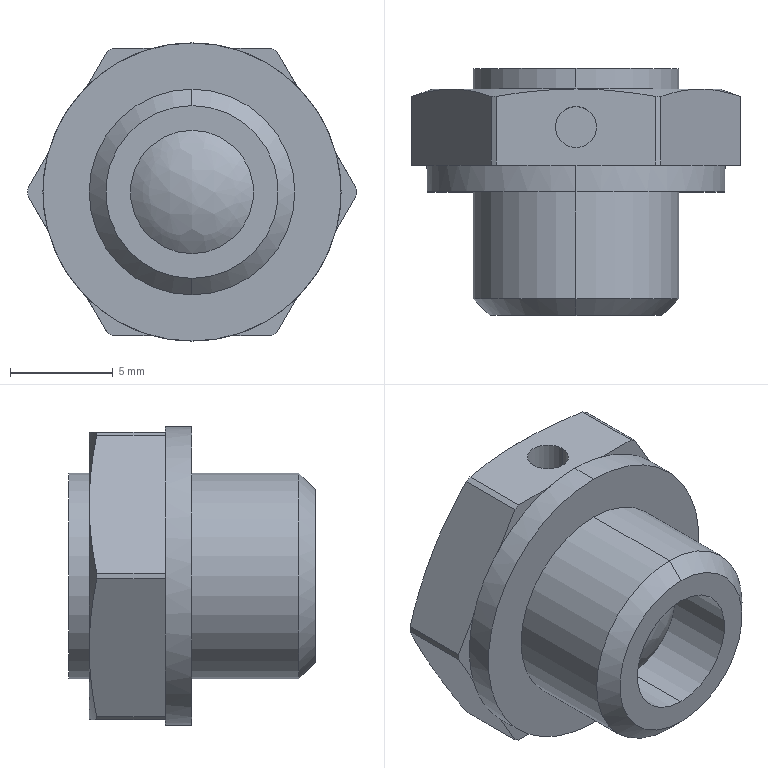Part | SolidWorks | features BaseBody 1 | 1 solid | 49 faces | box 16 x 12 x 14.5 mm | volume 1277 mm3 | plane 23 | cylinder 16 | cone 9 | spline 1 | commonest cylinder face diameters 16 x6 10 x4 2 x2 6 x2 14.5 x2
STEP:
#1=CARTESIAN_POINT('',(0.,0.,-5.));
#2=VERTEX_POINT('',#1);
#3=CARTESIAN_POINT('',(0.,0.,5.));
#4=VERTEX_POINT('',#3);
#5=CARTESIAN_POINT('',(0.,0.,0.));
#6=DIRECTION('',(0.,-1.,0.));
#7=DIRECTION('',(0.,0.,-1.));
#8=AXIS2_PLACEMENT_3D('',#5,#6,#7);
#9=CIRCLE('',#8,5.);
#10=EDGE_CURVE('',#2,#4,#9,.T.);
#11=ORIENTED_EDGE('',*,*,#10,.T.);
#12=CARTESIAN_POINT('',(0.,-5.2,5.));
#13=VERTEX_POINT('',#12);
#14=CARTESIAN_POINT('',(0.,-3.6,5.));
#15=DIRECTION('',(0.,-1.,0.));
#16=VECTOR('',#15,1000.);
#17=LINE('',#14,#16);
#18=EDGE_CURVE('',#4,#13,#17,.T.);
#19=ORIENTED_EDGE('',*,*,#18,.T.);
#20=CARTESIAN_POINT('',(0.,-5.2,-5.));
#21=VERTEX_POINT('',#20);
#22=CARTESIAN_POINT('',(0.,-5.2,0.));
#23=DIRECTION('',(0.,1.,0.));
#24=DIRECTION('',(0.,0.,-1.));
#25=AXIS2_PLACEMENT_3D('',#22,#23,#24);
#26=CIRCLE('',#25,5.);
#27=EDGE_CURVE('',#13,#21,#26,.T.);
#28=ORIENTED_EDGE('',*,*,#27,.T.);
#29=CARTESIAN_POINT('',(0.,-3.6,-5.));
#30=DIRECTION('',(0.,-1.,0.));
#31=VECTOR('',#30,1000.);
#32=LINE('',#29,#31);
#33=EDGE_CURVE('',#2,#21,#32,.T.);
#34=ORIENTED_EDGE('',*,*,#33,.F.);
#35=EDGE_LOOP('',(#11,#19,#28,#34));
#36=FACE_OUTER_BOUND('',#35,.T.);
#37=CARTESIAN_POINT('',(0.,-3.6,0.));
#38=DIRECTION('',(0.,-1.,0.));
#39=DIRECTION('',(0.,0.,-1.));
#40=AXIS2_PLACEMENT_3D('',#37,#38,#39);
#41=CYLINDRICAL_SURFACE('',#40,5.);
#42=ADVANCED_FACE('',(#36),#41,.T.);
#43=CARTESIAN_POINT('',(0.,-6.,4.2));
#44=VERTEX_POINT('',#43);
#45=CARTESIAN_POINT('',(0.,-6.,-4.2));
#46=VERTEX_POINT('',#45);
#47=CARTESIAN_POINT('',(0.,-6.,0.));
#48=DIRECTION('',(0.,1.,0.));
#49=DIRECTION('',(0.,0.,1.));
#50=AXIS2_PLACEMENT_3D('',#47,#48,#49);
#51=CIRCLE('',#50,4.2);
#52=EDGE_CURVE('',#44,#46,#51,.T.);
#53=ORIENTED_EDGE('',*,*,#52,.T.);
#54=CARTESIAN_POINT('',(0.,-5.2,-5.));
#55=DIRECTION('',(0.,0.7071,-0.7071));
#56=VECTOR('',#55,1000.);
#57=LINE('',#54,#56);
#58=EDGE_CURVE('',#46,#21,#57,.T.);
#59=ORIENTED_EDGE('',*,*,#58,.T.);
#60=ORIENTED_EDGE('',*,*,#27,.F.);
#61=CARTESIAN_POINT('',(0.,-5.2,5.));
#62=DIRECTION('',(0.,0.7071,0.7071));
#63=VECTOR('',#62,1000.);
#64=LINE('',#61,#63);
#65=EDGE_CURVE('',#44,#13,#64,.T.);
#66=ORIENTED_EDGE('',*,*,#65,.F.);
#67=EDGE_LOOP('',(#53,#59,#60,#66));
#68=FACE_OUTER_BOUND('',#67,.T.);
#69=CARTESIAN_POINT('',(0.,-5.2,0.));
#70=DIRECTION('',(0.,1.,0.));
#71=DIRECTION('',(0.,0.,1.));
#72=AXIS2_PLACEMENT_3D('',#69,#70,#71);
#73=CONICAL_SURFACE('',#72,5.,0.7854);
#74=ADVANCED_FACE('',(#68),#73,.T.);
#75=CARTESIAN_POINT('',(1.887,1.3,7.));
#76=VERTEX_POINT('',#75);
#77=CARTESIAN_POINT('',(0.,1.3,7.25));
#78=VERTEX_POINT('',#77);
#79=CARTESIAN_POINT('',(0.,1.3,0.));
#80=DIRECTION('',(0.,-1.,0.));
#81=DIRECTION('',(0.,0.,-1.));
#82=AXIS2_PLACEMENT_3D('',#79,#80,#81);
#83=CIRCLE('',#82,7.25);
#84=EDGE_CURVE('',#76,#78,#83,.T.);
#85=ORIENTED_EDGE('',*,*,#84,.T.);
#86=CARTESIAN_POINT('',(0.,0.,7.25));
#87=VERTEX_POINT('',#86);
#88=CARTESIAN_POINT('',(0.,-3.6,7.25));
#89=DIRECTION('',(0.,-1.,0.));
#90=VECTOR('',#89,1000.);
#91=LINE('',#88,#90);
#92=EDGE_CURVE('',#78,#87,#91,.T.);
#93=ORIENTED_EDGE('',*,*,#92,.T.);
#94=CARTESIAN_POINT('',(0.,0.,-7.25));
#95=VERTEX_POINT('',#94);
#96=CARTESIAN_POINT('',(0.,0.,0.));
#97=DIRECTION('',(0.,1.,0.));
#98=DIRECTION('',(0.,0.,-1.));
#99=AXIS2_PLACEMENT_3D('',#96,#97,#98);
#100=CIRCLE('',#99,7.25);
#101=EDGE_CURVE('',#87,#95,#100,.T.);
#102=ORIENTED_EDGE('',*,*,#101,.T.);
#103=CARTESIAN_POINT('',(0.,1.3,-7.25));
#104=VERTEX_POINT('',#103);
#105=CARTESIAN_POINT('',(0.,-3.6,-7.25));
#106=DIRECTION('',(0.,-1.,0.));
#107=VECTOR('',#106,1000.);
#108=LINE('',#105,#107);
#109=EDGE_CURVE('',#104,#95,#108,.T.);
#110=ORIENTED_EDGE('',*,*,#109,.F.);
#111=CARTESIAN_POINT('',(1.887,1.3,-7.));
#112=VERTEX_POINT('',#111);
#113=CARTESIAN_POINT('',(0.,1.3,0.));
#114=DIRECTION('',(0.,-1.,0.));
#115=DIRECTION('',(0.,0.,-1.));
#116=AXIS2_PLACEMENT_3D('',#113,#114,#115);
#117=CIRCLE('',#116,7.25);
#118=EDGE_CURVE('',#104,#112,#117,.T.);
#119=ORIENTED_EDGE('',*,*,#118,.T.);
#120=CARTESIAN_POINT('',(5.118,1.3,-5.135));
#121=VERTEX_POINT('',#120);
#122=CARTESIAN_POINT('',(0.,1.3,0.));
#123=DIRECTION('',(0.,-1.,0.));
#124=DIRECTION('',(0.,0.,-1.));
#125=AXIS2_PLACEMENT_3D('',#122,#123,#124);
#126=CIRCLE('',#125,7.25);
#127=EDGE_CURVE('',#112,#121,#126,.T.);
#128=ORIENTED_EDGE('',*,*,#127,.T.);
#129=CARTESIAN_POINT('',(7.006,1.3,-1.865));
#130=VERTEX_POINT('',#129);
#131=CARTESIAN_POINT('',(0.,1.3,0.));
#132=DIRECTION('',(0.,-1.,0.));
#133=DIRECTION('',(0.,0.,-1.));
#134=AXIS2_PLACEMENT_3D('',#131,#132,#133);
#135=CIRCLE('',#134,7.25);
#136=EDGE_CURVE('',#121,#130,#135,.T.);
#137=ORIENTED_EDGE('',*,*,#136,.T.);
#138=CARTESIAN_POINT('',(7.006,1.3,1.865));
#139=VERTEX_POINT('',#138);
#140=CARTESIAN_POINT('',(0.,1.3,0.));
#141=DIRECTION('',(0.,-1.,0.));
#142=DIRECTION('',(0.,0.,-1.));
#143=AXIS2_PLACEMENT_3D('',#140,#141,#142);
#144=CIRCLE('',#143,7.25);
#145=EDGE_CURVE('',#130,#139,#144,.T.);
#146=ORIENTED_EDGE('',*,*,#145,.T.);
#147=CARTESIAN_POINT('',(5.118,1.3,5.135));
#148=VERTEX_POINT('',#147);
#149=CARTESIAN_POINT('',(0.,1.3,0.));
#150=DIRECTION('',(0.,-1.,0.));
#151=DIRECTION('',(0.,0.,-1.));
#152=AXIS2_PLACEMENT_3D('',#149,#150,#151);
#153=CIRCLE('',#152,7.25);
#154=EDGE_CURVE('',#139,#148,#153,.T.);
#155=ORIENTED_EDGE('',*,*,#154,.T.);
#156=CARTESIAN_POINT('',(0.,1.3,0.));
#157=DIRECTION('',(0.,-1.,0.));
#158=DIRECTION('',(0.,0.,-1.));
#159=AXIS2_PLACEMENT_3D('',#156,#157,#158);
#160=CIRCLE('',#159,7.25);
#161=EDGE_CURVE('',#148,#76,#160,.T.);
#162=ORIENTED_EDGE('',*,*,#161,.T.);
#163=EDGE_LOOP('',(#85,#93,#102,#110,#119,#128,#137,#146,#155,#162));
#164=FACE_OUTER_BOUND('',#163,.T.);
#165=CARTESIAN_POINT('',(0.,-3.6,0.));
#166=DIRECTION('',(0.,-1.,0.));
#167=DIRECTION('',(0.,0.,-1.));
#168=AXIS2_PLACEMENT_3D('',#165,#166,#167);
#169=CYLINDRICAL_SURFACE('',#168,7.25);
#170=ADVANCED_FACE('',(#164),#169,.T.);
#171=CARTESIAN_POINT('',(0.,-2.6,3.));
#172=VERTEX_POINT('',#171);
#173=CARTESIAN_POINT('',(0.,-2.6,-3.));
#174=VERTEX_POINT('',#173);
#175=CARTESIAN_POINT('',(0.,-2.6,0.));
#176=DIRECTION('',(0.,-1.,0.));
#177=DIRECTION('',(0.,0.,-1.));
#178=AXIS2_PLACEMENT_3D('',#175,#176,#177);
#179=CIRCLE('',#178,3.);
#180=EDGE_CURVE('',#172,#174,#179,.T.);
#181=ORIENTED_EDGE('',*,*,#180,.F.);
#182=CARTESIAN_POINT('',(0.,-6.,3.));
#183=VERTEX_POINT('',#182);
#184=CARTESIAN_POINT('',(0.,-3.6,3.));
#185=DIRECTION('',(0.,-1.,0.));
#186=VECTOR('',#185,1000.);
#187=LINE('',#184,#186);
#188=EDGE_CURVE('',#172,#183,#187,.T.);
#189=ORIENTED_EDGE('',*,*,#188,.T.);
#190=CARTESIAN_POINT('',(0.,-6.,-3.));
#191=VERTEX_POINT('',#190);
#192=CARTESIAN_POINT('',(0.,-6.,0.));
#193=DIRECTION('',(0.,-1.,0.));
#194=DIRECTION('',(0.,0.,-1.));
#195=AXIS2_PLACEMENT_3D('',#192,#193,#194);
#196=CIRCLE('',#195,3.);
#197=EDGE_CURVE('',#183,#191,#196,.T.);
#198=ORIENTED_EDGE('',*,*,#197,.T.);
#199=CARTESIAN_POINT('',(0.,-3.6,-3.));
#200=DIRECTION('',(0.,-1.,0.));
#201=VECTOR('',#200,1000.);
#202=LINE('',#199,#201);
#203=EDGE_CURVE('',#174,#191,#202,.T.);
#204=ORIENTED_EDGE('',*,*,#203,.F.);
#205=EDGE_LOOP('',(#181,#189,#198,#204));
#206=FACE_OUTER_BOUND('',#205,.T.);
#207=CARTESIAN_POINT('',(0.,-3.6,0.));
#208=DIRECTION('',(0.,-1.,0.));
#209=DIRECTION('',(0.,0.,-1.));
#210=AXIS2_PLACEMENT_3D('',#207,#208,#209);
#211=CYLINDRICAL_SURFACE('',#210,3.);
#212=ADVANCED_FACE('',(#206),#211,.F.);
#213=CARTESIAN_POINT('',(6.062,5.,-3.5));
#214=VERTEX_POINT('',#213);
#215=CARTESIAN_POINT('',(7.,5.,0.));
#216=VERTEX_POINT('',#215);
#217=CARTESIAN_POINT('',(0.,5.,0.));
#218=DIRECTION('',(0.,-1.,0.));
#219=DIRECTION('',(1.,0.,0.));
#220=AXIS2_PLACEMENT_3D('',#217,#218,#219);
#221=CIRCLE('',#220,7.);
#222=EDGE_CURVE('',#214,#216,#221,.T.);
#223=ORIENTED_EDGE('',*,*,#222,.T.);
#224=CARTESIAN_POINT('',(8.,4.636,0.));
#225=VERTEX_POINT('',#224);
#226=CARTESIAN_POINT('',(8.,4.636,0.));
#227=DIRECTION('',(0.9397,-0.342,0.));
#228=VECTOR('',#227,1000.);
#229=LINE('',#226,#228);
#230=EDGE_CURVE('',#216,#225,#229,.T.);
#231=ORIENTED_EDGE('',*,*,#230,.T.);
#232=CARTESIAN_POINT('',(7.999,4.636,-0.1459));
#233=VERTEX_POINT('',#232);
#234=CARTESIAN_POINT('',(0.,4.636,0.));
#235=DIRECTION('',(0.,-1.,0.));
#236=DIRECTION('',(0.,0.,-1.));
#237=AXIS2_PLACEMENT_3D('',#234,#235,#236);
#238=CIRCLE('',#237,8.);
#239=EDGE_CURVE('',#233,#225,#238,.T.);
#240=ORIENTED_EDGE('',*,*,#239,.F.);
#241=CARTESIAN_POINT('',(7.999,4.636,-0.1459));
#242=CARTESIAN_POINT('',(7.358,4.862,-1.255));
#243=CARTESIAN_POINT('',(6.713,5.,-2.372));
#244=CARTESIAN_POINT('',(6.062,5.,-3.5));
#245=B_SPLINE_CURVE_WITH_KNOTS('',3,(#241,#242,#243,#244),.UNSPECIFIED.,.F.,.F.,(4,4),(0.,0.00389),.UNSPECIFIED.);
#246=EDGE_CURVE('',#233,#214,#245,.T.);
#247=ORIENTED_EDGE('',*,*,#246,.T.);
#248=EDGE_LOOP('',(#223,#231,#240,#247));
#249=FACE_OUTER_BOUND('',#248,.T.);
#250=CARTESIAN_POINT('',(0.,4.636,0.));
#251=DIRECTION('',(0.,-1.,0.));
#252=DIRECTION('',(1.,0.,0.));
#253=AXIS2_PLACEMENT_3D('',#250,#251,#252);
#254=CONICAL_SURFACE('',#253,8.,1.222);
#255=ADVANCED_FACE('',(#249),#254,.T.);
#256=CARTESIAN_POINT('',(-1.,3.15,7.));
#257=VERTEX_POINT('',#256);
#258=CARTESIAN_POINT('',(1.,3.15,7.));
#259=VERTEX_POINT('',#258);
#260=CARTESIAN_POINT('',(0.,3.15,7.));
#261=DIRECTION('',(0.,0.,1.));
#262=DIRECTION('',(-1.,0.,0.));
#263=AXIS2_PLACEMENT_3D('',#260,#261,#262);
#264=CIRCLE('',#263,1.);
#265=EDGE_CURVE('',#257,#259,#264,.T.);
#266=ORIENTED_EDGE('',*,*,#265,.T.);
#267=CARTESIAN_POINT('',(1.,3.15,0.));
#268=VERTEX_POINT('',#267);
#269=CARTESIAN_POINT('',(1.,3.15,0.));
#270=DIRECTION('',(0.,0.,-1.));
#271=VECTOR('',#270,1000.);
#272=LINE('',#269,#271);
#273=EDGE_CURVE('',#259,#268,#272,.T.);
#274=ORIENTED_EDGE('',*,*,#273,.T.);
#275=CARTESIAN_POINT('',(-1.,3.15,0.));
#276=VERTEX_POINT('',#275);
#277=CARTESIAN_POINT('',(0.,3.15,0.));
#278=DIRECTION('',(0.,0.,1.));
#279=DIRECTION('',(-1.,0.,0.));
#280=AXIS2_PLACEMENT_3D('',#277,#278,#279);
#281=CIRCLE('',#280,1.);
#282=EDGE_CURVE('',#276,#268,#281,.T.);
#283=ORIENTED_EDGE('',*,*,#282,.F.);
#284=CARTESIAN_POINT('',(-1.,3.15,0.));
#285=DIRECTION('',(0.,0.,-1.));
#286=VECTOR('',#285,1000.);
#287=LINE('',#284,#286);
#288=EDGE_CURVE('',#257,#276,#287,.T.);
#289=ORIENTED_EDGE('',*,*,#288,.F.);
#290=EDGE_LOOP('',(#266,#274,#283,#289));
#291=FACE_OUTER_BOUND('',#290,.T.);
#292=CARTESIAN_POINT('',(0.,3.15,0.));
#293=DIRECTION('',(0.,0.,-1.));
#294=DIRECTION('',(-1.,0.,0.));
#295=AXIS2_PLACEMENT_3D('',#292,#293,#294);
#296=CYLINDRICAL_SURFACE('',#295,1.);
#297=ADVANCED_FACE('',(#291),#296,.F.);
#298=CARTESIAN_POINT('',(0.,6.,-5.));
#299=VERTEX_POINT('',#298);
#300=CARTESIAN_POINT('',(0.,6.,5.));
#301=VERTEX_POINT('',#300);
#302=CARTESIAN_POINT('',(0.,6.,0.));
#303=DIRECTION('',(0.,-1.,0.));
#304=DIRECTION('',(0.,0.,-1.));
#305=AXIS2_PLACEMENT_3D('',#302,#303,#304);
#306=CIRCLE('',#305,5.);
#307=EDGE_CURVE('',#299,#301,#306,.T.);
#308=ORIENTED_EDGE('',*,*,#307,.T.);
#309=CARTESIAN_POINT('',(0.,5.,5.));
#310=VERTEX_POINT('',#309);
#311=CARTESIAN_POINT('',(0.,-3.6,5.));
#312=DIRECTION('',(0.,-1.,0.));
#313=VECTOR('',#312,1000.);
#314=LINE('',#311,#313);
#315=EDGE_CURVE('',#301,#310,#314,.T.);
#316=ORIENTED_EDGE('',*,*,#315,.T.);
#317=CARTESIAN_POINT('',(0.,5.,-5.));
#318=VERTEX_POINT('',#317);
#319=CARTESIAN_POINT('',(0.,5.,0.));
#320=DIRECTION('',(0.,1.,0.));
#321=DIRECTION('',(0.,0.,-1.));
#322=AXIS2_PLACEMENT_3D('',#319,#320,#321);
#323=CIRCLE('',#322,5.);
#324=EDGE_CURVE('',#310,#318,#323,.T.);
#325=ORIENTED_EDGE('',*,*,#324,.T.);
#326=CARTESIAN_POINT('',(0.,-3.6,-5.));
#327=DIRECTION('',(0.,-1.,0.));
#328=VECTOR('',#327,1000.);
#329=LINE('',#326,#328);
#330=EDGE_CURVE('',#299,#318,#329,.T.);
#331=ORIENTED_EDGE('',*,*,#330,.F.);
#332=EDGE_LOOP('',(#308,#316,#325,#331));
#333=FACE_OUTER_BOUND('',#332,.T.);
#334=CARTESIAN_POINT('',(0.,-3.6,0.));
#335=DIRECTION('',(0.,-1.,0.));
#336=DIRECTION('',(0.,0.,-1.));
#337=AXIS2_PLACEMENT_3D('',#334,#335,#336);
#338=CYLINDRICAL_SURFACE('',#337,5.);
#339=ADVANCED_FACE('',(#333),#338,.T.);
#340=ORIENTED_EDGE('',*,*,#18,.F.);
#341=CARTESIAN_POINT('',(0.,0.,0.));
#342=DIRECTION('',(0.,-1.,0.));
#343=DIRECTION('',(0.,0.,-1.));
#344=AXIS2_PLACEMENT_3D('',#341,#342,#343);
#345=CIRCLE('',#344,5.);
#346=EDGE_CURVE('',#4,#2,#345,.T.);
#347=ORIENTED_EDGE('',*,*,#346,.T.);
#348=ORIENTED_EDGE('',*,*,#33,.T.);
#349=CARTESIAN_POINT('',(0.,-5.2,0.));
#350=DIRECTION('',(0.,1.,0.));
#351=DIRECTION('',(0.,0.,-1.));
#352=AXIS2_PLACEMENT_3D('',#349,#350,#351);
#353=CIRCLE('',#352,5.);
#354=EDGE_CURVE('',#21,#13,#353,.T.);
#355=ORIENTED_EDGE('',*,*,#354,.T.);
#356=EDGE_LOOP('',(#340,#347,#348,#355));
#357=FACE_OUTER_BOUND('',#356,.T.);
#358=CARTESIAN_POINT('',(0.,-3.6,0.));
#359=DIRECTION('',(0.,-1.,0.));
#360=DIRECTION('',(0.,0.,-1.));
#361=AXIS2_PLACEMENT_3D('',#358,#359,#360);
#362=CYLINDRICAL_SURFACE('',#361,5.);
#363=ADVANCED_FACE('',(#357),#362,.T.);
#364=CARTESIAN_POINT('',(0.,0.,0.));
#365=DIRECTION('',(0.,1.,0.));
#366=DIRECTION('',(0.,0.,-1.));
#367=AXIS2_PLACEMENT_3D('',#364,#365,#366);
#368=CIRCLE('',#367,7.25);
#369=EDGE_CURVE('',#95,#87,#368,.T.);
#370=ORIENTED_EDGE('',*,*,#369,.F.);
#371=ORIENTED_EDGE('',*,*,#101,.F.);
#372=EDGE_LOOP('',(#370,#371));
#373=FACE_OUTER_BOUND('',#372,.T.);
#374=ORIENTED_EDGE('',*,*,#10,.F.);
#375=ORIENTED_EDGE('',*,*,#346,.F.);
#376=EDGE_LOOP('',(#374,#375));
#377=FACE_BOUND('',#376,.T.);
#378=CARTESIAN_POINT('',(7.25,0.,0.));
#379=DIRECTION('',(0.,1.,0.));
#380=DIRECTION('',(0.,0.,1.));
#381=AXIS2_PLACEMENT_3D('',#378,#379,#380);
#382=PLANE('',#381);
#383=ADVANCED_FACE('',(#373,#377),#382,.F.);
#384=ORIENTED_EDGE('',*,*,#58,.F.);
#385=CARTESIAN_POINT('',(0.,-6.,0.));
#386=DIRECTION('',(0.,1.,0.));
#387=DIRECTION('',(0.,0.,1.));
#388=AXIS2_PLACEMENT_3D('',#385,#386,#387);
#389=CIRCLE('',#388,4.2);
#390=EDGE_CURVE('',#46,#44,#389,.T.);
#391=ORIENTED_EDGE('',*,*,#390,.T.);
#392=ORIENTED_EDGE('',*,*,#65,.T.);
#393=ORIENTED_EDGE('',*,*,#354,.F.);
#394=EDGE_LOOP('',(#384,#391,#392,#393));
#395=FACE_OUTER_BOUND('',#394,.T.);
#396=CARTESIAN_POINT('',(0.,-5.2,0.));
#397=DIRECTION('',(0.,1.,0.));
#398=DIRECTION('',(0.,0.,1.));
#399=AXIS2_PLACEMENT_3D('',#396,#397,#398);
#400=CONICAL_SURFACE('',#399,5.,0.7854);
#401=ADVANCED_FACE('',(#395),#400,.T.);
#402=ORIENTED_EDGE('',*,*,#92,.F.);
#403=CARTESIAN_POINT('',(-1.887,1.3,7.));
#404=VERTEX_POINT('',#403);
#405=CARTESIAN_POINT('',(0.,1.3,0.));
#406=DIRECTION('',(0.,-1.,0.));
#407=DIRECTION('',(0.,0.,-1.));
#408=AXIS2_PLACEMENT_3D('',#405,#406,#407);
#409=CIRCLE('',#408,7.25);
#410=EDGE_CURVE('',#78,#404,#409,.T.);
#411=ORIENTED_EDGE('',*,*,#410,.T.);
#412=CARTESIAN_POINT('',(-5.118,1.3,5.135));
#413=VERTEX_POINT('',#412);
#414=CARTESIAN_POINT('',(0.,1.3,0.));
#415=DIRECTION('',(0.,-1.,0.));
#416=DIRECTION('',(0.,0.,-1.));
#417=AXIS2_PLACEMENT_3D('',#414,#415,#416);
#418=CIRCLE('',#417,7.25);
#419=EDGE_CURVE('',#404,#413,#418,.T.);
#420=ORIENTED_EDGE('',*,*,#419,.T.);
#421=CARTESIAN_POINT('',(-7.006,1.3,1.865));
#422=VERTEX_POINT('',#421);
#423=CARTESIAN_POINT('',(0.,1.3,0.));
#424=DIRECTION('',(0.,-1.,0.));
#425=DIRECTION('',(0.,0.,-1.));
#426=AXIS2_PLACEMENT_3D('',#423,#424,#425);
#427=CIRCLE('',#426,7.25);
#428=EDGE_CURVE('',#413,#422,#427,.T.);
#429=ORIENTED_EDGE('',*,*,#428,.T.);
#430=CARTESIAN_POINT('',(-7.006,1.3,-1.865));
#431=VERTEX_POINT('',#430);
#432=CARTESIAN_POINT('',(0.,1.3,0.));
#433=DIRECTION('',(0.,-1.,0.));
#434=DIRECTION('',(0.,0.,-1.));
#435=AXIS2_PLACEMENT_3D('',#432,#433,#434);
#436=CIRCLE('',#435,7.25);
#437=EDGE_CURVE('',#422,#431,#436,.T.);
#438=ORIENTED_EDGE('',*,*,#437,.T.);
#439=CARTESIAN_POINT('',(-5.118,1.3,-5.135));
#440=VERTEX_POINT('',#439);
#441=CARTESIAN_POINT('',(0.,1.3,0.));
#442=DIRECTION('',(0.,-1.,0.));
#443=DIRECTION('',(0.,0.,-1.));
#444=AXIS2_PLACEMENT_3D('',#441,#442,#443);
#445=CIRCLE('',#444,7.25);
#446=EDGE_CURVE('',#431,#440,#445,.T.);
#447=ORIENTED_EDGE('',*,*,#446,.T.);
#448=CARTESIAN_POINT('',(-1.887,1.3,-7.));
#449=VERTEX_POINT('',#448);
#450=CARTESIAN_POINT('',(0.,1.3,0.));
#451=DIRECTION('',(0.,-1.,0.));
#452=DIRECTION('',(0.,0.,-1.));
#453=AXIS2_PLACEMENT_3D('',#450,#451,#452);
#454=CIRCLE('',#453,7.25);
#455=EDGE_CURVE('',#440,#449,#454,.T.);
#456=ORIENTED_EDGE('',*,*,#455,.T.);
#457=CARTESIAN_POINT('',(0.,1.3,0.));
#458=DIRECTION('',(0.,-1.,0.));
#459=DIRECTION('',(0.,0.,-1.));
#460=AXIS2_PLACEMENT_3D('',#457,#458,#459);
#461=CIRCLE('',#460,7.25);
#462=EDGE_CURVE('',#449,#104,#461,.T.);
#463=ORIENTED_EDGE('',*,*,#462,.T.);
#464=ORIENTED_EDGE('',*,*,#109,.T.);
#465=ORIENTED_EDGE('',*,*,#369,.T.);
#466=EDGE_LOOP('',(#402,#411,#420,#429,#438,#447,#456,#463,#464,#465));
#467=FACE_OUTER_BOUND('',#466,.T.);
#468=CARTESIAN_POINT('',(0.,-3.6,0.));
#469=DIRECTION('',(0.,-1.,0.));
#470=DIRECTION('',(0.,0.,-1.));
#471=AXIS2_PLACEMENT_3D('',#468,#469,#470);
#472=CYLINDRICAL_SURFACE('',#471,7.25);
#473=ADVANCED_FACE('',(#467),#472,.T.);
#474=ORIENTED_EDGE('',*,*,#52,.F.);
#475=ORIENTED_EDGE('',*,*,#390,.F.);
#476=EDGE_LOOP('',(#474,#475));
#477=FACE_OUTER_BOUND('',#476,.T.);
#478=CARTESIAN_POINT('',(0.,-6.,0.));
#479=DIRECTION('',(0.,-1.,0.));
#480=DIRECTION('',(0.,0.,-1.));
#481=AXIS2_PLACEMENT_3D('',#478,#479,#480);
#482=CIRCLE('',#481,3.);
#483=EDGE_CURVE('',#191,#183,#482,.T.);
#484=ORIENTED_EDGE('',*,*,#483,.F.);
#485=ORIENTED_EDGE('',*,*,#197,.F.);
#486=EDGE_LOOP('',(#484,#485));
#487=FACE_BOUND('',#486,.T.);
#488=CARTESIAN_POINT('',(4.2,-6.,0.));
#489=DIRECTION('',(0.,1.,0.));
#490=DIRECTION('',(0.,0.,1.));
#491=AXIS2_PLACEMENT_3D('',#488,#489,#490);
#492=PLANE('',#491);
#493=ADVANCED_FACE('',(#477,#487),#492,.F.);
#494=CARTESIAN_POINT('',(3.873,1.3,-7.));
#495=VERTEX_POINT('',#494);
#496=CARTESIAN_POINT('',(8.4,1.3,-7.));
#497=DIRECTION('',(-1.,0.,0.));
#498=VECTOR('',#497,1000.);
#499=LINE('',#496,#498);
#500=EDGE_CURVE('',#495,#112,#499,.T.);
#501=ORIENTED_EDGE('',*,*,#500,.F.);
#502=CARTESIAN_POINT('',(4.126,1.3,-6.854));
#503=VERTEX_POINT('',#502);
#504=CARTESIAN_POINT('',(0.,1.3,0.));
#505=DIRECTION('',(0.,1.,0.));
#506=DIRECTION('',(0.,0.,-1.));
#507=AXIS2_PLACEMENT_3D('',#504,#505,#506);
#508=CIRCLE('',#507,8.);
#509=EDGE_CURVE('',#503,#495,#508,.T.);
#510=ORIENTED_EDGE('',*,*,#509,.F.);
#511=CARTESIAN_POINT('',(5.118,1.3,-5.135));
#512=DIRECTION('',(-0.5,0.,-0.866));
#513=VECTOR('',#512,1000.);
#514=LINE('',#511,#513);
#515=EDGE_CURVE('',#121,#503,#514,.T.);
#516=ORIENTED_EDGE('',*,*,#515,.F.);
#517=ORIENTED_EDGE('',*,*,#127,.F.);
#518=EDGE_LOOP('',(#501,#510,#516,#517));
#519=FACE_OUTER_BOUND('',#518,.T.);
#520=CARTESIAN_POINT('',(8.4,1.3,0.));
#521=DIRECTION('',(0.,1.,0.));
#522=DIRECTION('',(0.,0.,1.));
#523=AXIS2_PLACEMENT_3D('',#520,#521,#522);
#524=PLANE('',#523);
#525=ADVANCED_FACE('',(#519),#524,.F.);
#526=ORIENTED_EDGE('',*,*,#462,.F.);
#527=CARTESIAN_POINT('',(0.,1.3,-7.));
#528=DIRECTION('',(1.,0.,0.));
#529=VECTOR('',#528,1000.);
#530=LINE('',#527,#529);
#531=EDGE_CURVE('',#449,#112,#530,.T.);
#532=ORIENTED_EDGE('',*,*,#531,.T.);
#533=ORIENTED_EDGE('',*,*,#118,.F.);
#534=EDGE_LOOP('',(#526,#532,#533));
#535=FACE_OUTER_BOUND('',#534,.T.);
#536=CARTESIAN_POINT('',(0.,1.3,0.));
#537=DIRECTION('',(0.,1.,0.));
#538=DIRECTION('',(0.,0.,1.));
#539=AXIS2_PLACEMENT_3D('',#536,#537,#538);
#540=PLANE('',#539);
#541=ADVANCED_FACE('',(#535),#540,.T.);
#542=CARTESIAN_POINT('',(-4.126,1.3,-6.854));
#543=VERTEX_POINT('',#542);
#544=CARTESIAN_POINT('',(-4.126,1.3,-6.854));
#545=DIRECTION('',(-0.5,0.,0.866));
#546=VECTOR('',#545,1000.);
#547=LINE('',#544,#546);
#548=EDGE_CURVE('',#543,#440,#547,.T.);
#549=ORIENTED_EDGE('',*,*,#548,.F.);
#550=CARTESIAN_POINT('',(-3.873,1.3,-7.));
#551=VERTEX_POINT('',#550);
#552=CARTESIAN_POINT('',(0.,1.3,0.));
#553=DIRECTION('',(0.,1.,0.));
#554=DIRECTION('',(0.,0.,-1.));
#555=AXIS2_PLACEMENT_3D('',#552,#553,#554);
#556=CIRCLE('',#555,8.);
#557=EDGE_CURVE('',#551,#543,#556,.T.);
#558=ORIENTED_EDGE('',*,*,#557,.F.);
#559=CARTESIAN_POINT('',(8.4,1.3,-7.));
#560=DIRECTION('',(-1.,0.,0.));
#561=VECTOR('',#560,1000.);
#562=LINE('',#559,#561);
#563=EDGE_CURVE('',#449,#551,#562,.T.);
#564=ORIENTED_EDGE('',*,*,#563,.F.);
#565=ORIENTED_EDGE('',*,*,#455,.F.);
#566=EDGE_LOOP('',(#549,#558,#564,#565));
#567=FACE_OUTER_BOUND('',#566,.T.);
#568=CARTESIAN_POINT('',(8.4,1.3,0.));
#569=DIRECTION('',(0.,1.,0.));
#570=DIRECTION('',(0.,0.,1.));
#571=AXIS2_PLACEMENT_3D('',#568,#569,#570);
#572=PLANE('',#571);
#573=ADVANCED_FACE('',(#567),#572,.F.);
#574=ORIENTED_EDGE('',*,*,#446,.F.);
#575=CARTESIAN_POINT('',(-7.006,1.3,-1.865));
#576=DIRECTION('',(0.5,0.,-0.866));
#577=VECTOR('',#576,1000.);
#578=LINE('',#575,#577);
#579=EDGE_CURVE('',#431,#440,#578,.T.);
#580=ORIENTED_EDGE('',*,*,#579,.T.);
#581=EDGE_LOOP('',(#574,#580));
#582=FACE_OUTER_BOUND('',#581,.T.);
#583=CARTESIAN_POINT('',(0.,1.3,0.));
#584=DIRECTION('',(0.,1.,0.));
#585=DIRECTION('',(0.,0.,1.));
#586=AXIS2_PLACEMENT_3D('',#583,#584,#585);
#587=PLANE('',#586);
#588=ADVANCED_FACE('',(#582),#587,.T.);
#589=CARTESIAN_POINT('',(-7.999,1.3,-0.1459));
#590=VERTEX_POINT('',#589);
#591=CARTESIAN_POINT('',(-7.006,1.3,-1.865));
#592=DIRECTION('',(-0.5,0.,0.866));
#593=VECTOR('',#592,1000.);
#594=LINE('',#591,#593);
#595=EDGE_CURVE('',#431,#590,#594,.T.);
#596=ORIENTED_EDGE('',*,*,#595,.F.);
#597=ORIENTED_EDGE('',*,*,#437,.F.);
#598=CARTESIAN_POINT('',(-7.999,1.3,0.1459));
#599=VERTEX_POINT('',#598);
#600=CARTESIAN_POINT('',(-7.999,1.3,0.1459));
#601=DIRECTION('',(0.5,0.,0.866));
#602=VECTOR('',#601,1000.);
#603=LINE('',#600,#602);
#604=EDGE_CURVE('',#599,#422,#603,.T.);
#605=ORIENTED_EDGE('',*,*,#604,.F.);
#606=CARTESIAN_POINT('',(0.,1.3,0.));
#607=DIRECTION('',(0.,1.,0.));
#608=DIRECTION('',(0.,0.,-1.));
#609=AXIS2_PLACEMENT_3D('',#606,#607,#608);
#610=CIRCLE('',#609,8.);
#611=EDGE_CURVE('',#590,#599,#610,.T.);
#612=ORIENTED_EDGE('',*,*,#611,.F.);
#613=EDGE_LOOP('',(#596,#597,#605,#612));
#614=FACE_OUTER_BOUND('',#613,.T.);
#615=CARTESIAN_POINT('',(8.4,1.3,0.));
#616=DIRECTION('',(0.,1.,0.));
#617=DIRECTION('',(0.,0.,1.));
#618=AXIS2_PLACEMENT_3D('',#615,#616,#617);
#619=PLANE('',#618);
#620=ADVANCED_FACE('',(#614),#619,.F.);
#621=ORIENTED_EDGE('',*,*,#428,.F.);
#622=CARTESIAN_POINT('',(-5.118,1.3,5.135));
#623=DIRECTION('',(-0.5,0.,-0.866));
#624=VECTOR('',#623,1000.);
#625=LINE('',#622,#624);
#626=EDGE_CURVE('',#413,#422,#625,.T.);
#627=ORIENTED_EDGE('',*,*,#626,.T.);
#628=EDGE_LOOP('',(#621,#627));
#629=FACE_OUTER_BOUND('',#628,.T.);
#630=CARTESIAN_POINT('',(0.,1.3,0.));
#631=DIRECTION('',(0.,1.,0.));
#632=DIRECTION('',(0.,0.,1.));
#633=AXIS2_PLACEMENT_3D('',#630,#631,#632);
#634=PLANE('',#633);
#635=ADVANCED_FACE('',(#629),#634,.T.);
#636=CARTESIAN_POINT('',(-3.873,1.3,7.));
#637=VERTEX_POINT('',#636);
#638=CARTESIAN_POINT('',(8.4,1.3,7.));
#639=DIRECTION('',(1.,0.,0.));
#640=VECTOR('',#639,1000.);
#641=LINE('',#638,#640);
#642=EDGE_CURVE('',#637,#404,#641,.T.);
#643=ORIENTED_EDGE('',*,*,#642,.F.);
#644=CARTESIAN_POINT('',(-4.126,1.3,6.854));
#645=VERTEX_POINT('',#644);
#646=CARTESIAN_POINT('',(0.,1.3,0.));
#647=DIRECTION('',(0.,1.,0.));
#648=DIRECTION('',(0.,0.,-1.));
#649=AXIS2_PLACEMENT_3D('',#646,#647,#648);
#650=CIRCLE('',#649,8.);
#651=EDGE_CURVE('',#645,#637,#650,.T.);
#652=ORIENTED_EDGE('',*,*,#651,.F.);
#653=CARTESIAN_POINT('',(-5.118,1.3,5.135));
#654=DIRECTION('',(0.5,0.,0.866));
#655=VECTOR('',#654,1000.);
#656=LINE('',#653,#655);
#657=EDGE_CURVE('',#413,#645,#656,.T.);
#658=ORIENTED_EDGE('',*,*,#657,.F.);
#659=ORIENTED_EDGE('',*,*,#419,.F.);
#660=EDGE_LOOP('',(#643,#652,#658,#659));
#661=FACE_OUTER_BOUND('',#660,.T.);
#662=CARTESIAN_POINT('',(8.4,1.3,0.));
#663=DIRECTION('',(0.,1.,0.));
#664=DIRECTION('',(0.,0.,1.));
#665=AXIS2_PLACEMENT_3D('',#662,#663,#664);
#666=PLANE('',#665);
#667=ADVANCED_FACE('',(#661),#666,.F.);
#668=ORIENTED_EDGE('',*,*,#84,.F.);
#669=CARTESIAN_POINT('',(0.,1.3,7.));
#670=DIRECTION('',(-1.,0.,0.));
#671=VECTOR('',#670,1000.);
#672=LINE('',#669,#671);
#673=EDGE_CURVE('',#76,#404,#672,.T.);
#674=ORIENTED_EDGE('',*,*,#673,.T.);
#675=ORIENTED_EDGE('',*,*,#410,.F.);
#676=EDGE_LOOP('',(#668,#674,#675));
#677=FACE_OUTER_BOUND('',#676,.T.);
#678=CARTESIAN_POINT('',(0.,1.3,0.));
#679=DIRECTION('',(0.,1.,0.));
#680=DIRECTION('',(0.,0.,1.));
#681=AXIS2_PLACEMENT_3D('',#678,#679,#680);
#682=PLANE('',#681);
#683=ADVANCED_FACE('',(#677),#682,.T.);
#684=CARTESIAN_POINT('',(4.126,1.3,6.854));
#685=VERTEX_POINT('',#684);
#686=CARTESIAN_POINT('',(4.126,1.3,6.854));
#687=DIRECTION('',(0.5,0.,-0.866));
#688=VECTOR('',#687,1000.);
#689=LINE('',#686,#688);
#690=EDGE_CURVE('',#685,#148,#689,.T.);
#691=ORIENTED_EDGE('',*,*,#690,.F.);
#692=CARTESIAN_POINT('',(3.873,1.3,7.));
#693=VERTEX_POINT('',#692);
#694=CARTESIAN_POINT('',(0.,1.3,0.));
#695=DIRECTION('',(0.,1.,0.));
#696=DIRECTION('',(0.,0.,-1.));
#697=AXIS2_PLACEMENT_3D('',#694,#695,#696);
#698=CIRCLE('',#697,8.);
#699=EDGE_CURVE('',#693,#685,#698,.T.);
#700=ORIENTED_EDGE('',*,*,#699,.F.);
#701=CARTESIAN_POINT('',(8.4,1.3,7.));
#702=DIRECTION('',(1.,0.,0.));
#703=VECTOR('',#702,1000.);
#704=LINE('',#701,#703);
#705=EDGE_CURVE('',#76,#693,#704,.T.);
#706=ORIENTED_EDGE('',*,*,#705,.F.);
#707=ORIENTED_EDGE('',*,*,#161,.F.);
#708=EDGE_LOOP('',(#691,#700,#706,#707));
#709=FACE_OUTER_BOUND('',#708,.T.);
#710=CARTESIAN_POINT('',(8.4,1.3,0.));
#711=DIRECTION('',(0.,1.,0.));
#712=DIRECTION('',(0.,0.,1.));
#713=AXIS2_PLACEMENT_3D('',#710,#711,#712);
#714=PLANE('',#713);
#715=ADVANCED_FACE('',(#709),#714,.F.);
#716=ORIENTED_EDGE('',*,*,#154,.F.);
#717=CARTESIAN_POINT('',(7.006,1.3,1.865));
#718=DIRECTION('',(-0.5,0.,0.866));
#719=VECTOR('',#718,1000.);
#720=LINE('',#717,#719);
#721=EDGE_CURVE('',#139,#148,#720,.T.);
#722=ORIENTED_EDGE('',*,*,#721,.T.);
#723=EDGE_LOOP('',(#716,#722));
#724=FACE_OUTER_BOUND('',#723,.T.);
#725=CARTESIAN_POINT('',(0.,1.3,0.));
#726=DIRECTION('',(0.,1.,0.));
#727=DIRECTION('',(0.,0.,1.));
#728=AXIS2_PLACEMENT_3D('',#725,#726,#727);
#729=PLANE('',#728);
#730=ADVANCED_FACE('',(#724),#729,.T.);
#731=CARTESIAN_POINT('',(7.999,1.3,-0.1459));
#732=VERTEX_POINT('',#731);
#733=CARTESIAN_POINT('',(7.999,1.3,-0.1459));
#734=DIRECTION('',(-0.5,0.,-0.866));
#735=VECTOR('',#734,1000.);
#736=LINE('',#733,#735);
#737=EDGE_CURVE('',#732,#130,#736,.T.);
#738=ORIENTED_EDGE('',*,*,#737,.F.);
#739=CARTESIAN_POINT('',(7.999,1.3,0.1459));
#740=VERTEX_POINT('',#739);
#741=CARTESIAN_POINT('',(0.,1.3,0.));
#742=DIRECTION('',(0.,1.,0.));
#743=DIRECTION('',(0.,0.,-1.));
#744=AXIS2_PLACEMENT_3D('',#741,#742,#743);
#745=CIRCLE('',#744,8.);
#746=EDGE_CURVE('',#740,#732,#745,.T.);
#747=ORIENTED_EDGE('',*,*,#746,.F.);
#748=CARTESIAN_POINT('',(7.006,1.3,1.865));
#749=DIRECTION('',(0.5,0.,-0.866));
#750=VECTOR('',#749,1000.);
#751=LINE('',#748,#750);
#752=EDGE_CURVE('',#139,#740,#751,.T.);
#753=ORIENTED_EDGE('',*,*,#752,.F.);
#754=ORIENTED_EDGE('',*,*,#145,.F.);
#755=EDGE_LOOP('',(#738,#747,#753,#754));
#756=FACE_OUTER_BOUND('',#755,.T.);
#757=CARTESIAN_POINT('',(8.4,1.3,0.));
#758=DIRECTION('',(0.,1.,0.));
#759=DIRECTION('',(0.,0.,1.));
#760=AXIS2_PLACEMENT_3D('',#757,#758,#759);
#761=PLANE('',#760);
#762=ADVANCED_FACE('',(#756),#761,.F.);
#763=ORIENTED_EDGE('',*,*,#136,.F.);
#764=CARTESIAN_POINT('',(5.118,1.3,-5.135));
#765=DIRECTION('',(0.5,0.,0.866));
#766=VECTOR('',#765,1000.);
#767=LINE('',#764,#766);
#768=EDGE_CURVE('',#121,#130,#767,.T.);
#769=ORIENTED_EDGE('',*,*,#768,.T.);
#770=EDGE_LOOP('',(#763,#769));
#771=FACE_OUTER_BOUND('',#770,.T.);
#772=CARTESIAN_POINT('',(0.,1.3,0.));
#773=DIRECTION('',(0.,1.,0.));
#774=DIRECTION('',(0.,0.,1.));
#775=AXIS2_PLACEMENT_3D('',#772,#773,#774);
#776=PLANE('',#775);
#777=ADVANCED_FACE('',(#771),#776,.T.);
#778=ORIENTED_EDGE('',*,*,#188,.F.);
#779=CARTESIAN_POINT('',(0.,-2.6,0.));
#780=DIRECTION('',(0.,-1.,0.));
#781=DIRECTION('',(0.,0.,-1.));
#782=AXIS2_PLACEMENT_3D('',#779,#780,#781);
#783=CIRCLE('',#782,3.);
#784=EDGE_CURVE('',#174,#172,#783,.T.);
#785=ORIENTED_EDGE('',*,*,#784,.F.);
#786=ORIENTED_EDGE('',*,*,#203,.T.);
#787=ORIENTED_EDGE('',*,*,#483,.T.);
#788=EDGE_LOOP('',(#778,#785,#786,#787));
#789=FACE_OUTER_BOUND('',#788,.T.);
#790=CARTESIAN_POINT('',(0.,-3.6,0.));
#791=DIRECTION('',(0.,-1.,0.));
#792=DIRECTION('',(0.,0.,-1.));
#793=AXIS2_PLACEMENT_3D('',#790,#791,#792);
#794=CYLINDRICAL_SURFACE('',#793,3.);
#795=ADVANCED_FACE('',(#789),#794,.F.);
#796=ORIENTED_EDGE('',*,*,#500,.T.);
#797=ORIENTED_EDGE('',*,*,#531,.F.);
#798=ORIENTED_EDGE('',*,*,#563,.T.);
#799=CARTESIAN_POINT('',(-3.873,4.636,-7.));
#800=VERTEX_POINT('',#799);
#801=CARTESIAN_POINT('',(-3.873,7.3,-7.));
#802=DIRECTION('',(0.,-1.,0.));
#803=VECTOR('',#802,1000.);
#804=LINE('',#801,#803);
#805=EDGE_CURVE('',#800,#551,#804,.T.);
#806=ORIENTED_EDGE('',*,*,#805,.F.);
#807=CARTESIAN_POINT('',(0.,5.,-7.));
#808=VERTEX_POINT('',#807);
#809=CARTESIAN_POINT('',(0.,5.,-7.));
#810=CARTESIAN_POINT('',(-1.302,5.,-7.));
#811=CARTESIAN_POINT('',(-2.592,4.862,-7.));
#812=CARTESIAN_POINT('',(-3.873,4.636,-7.));
#813=B_SPLINE_CURVE_WITH_KNOTS('',3,(#809,#810,#811,#812),.UNSPECIFIED.,.F.,.F.,(4,4),(0.,0.00389),.UNSPECIFIED.);
#814=EDGE_CURVE('',#808,#800,#813,.T.);
#815=ORIENTED_EDGE('',*,*,#814,.F.);
#816=CARTESIAN_POINT('',(3.873,4.636,-7.));
#817=VERTEX_POINT('',#816);
#818=CARTESIAN_POINT('',(3.873,4.636,-7.));
#819=CARTESIAN_POINT('',(2.592,4.862,-7.));
#820=CARTESIAN_POINT('',(1.302,5.,-7.));
#821=CARTESIAN_POINT('',(0.,5.,-7.));
#822=B_SPLINE_CURVE_WITH_KNOTS('',3,(#818,#819,#820,#821),.UNSPECIFIED.,.F.,.F.,(4,4),(0.,0.00389),.UNSPECIFIED.);
#823=EDGE_CURVE('',#817,#808,#822,.T.);
#824=ORIENTED_EDGE('',*,*,#823,.F.);
#825=CARTESIAN_POINT('',(3.873,7.3,-7.));
#826=DIRECTION('',(0.,1.,0.));
#827=VECTOR('',#826,1000.);
#828=LINE('',#825,#827);
#829=EDGE_CURVE('',#495,#817,#828,.T.);
#830=ORIENTED_EDGE('',*,*,#829,.F.);
#831=EDGE_LOOP('',(#796,#797,#798,#806,#815,#824,#830));
#832=FACE_OUTER_BOUND('',#831,.T.);
#833=CARTESIAN_POINT('',(3.873,7.3,-7.));
#834=DIRECTION('',(0.,0.,1.));
#835=DIRECTION('',(1.,0.,0.));
#836=AXIS2_PLACEMENT_3D('',#833,#834,#835);
#837=PLANE('',#836);
#838=ADVANCED_FACE('',(#832),#837,.F.);
#839=ORIENTED_EDGE('',*,*,#737,.T.);
#840=ORIENTED_EDGE('',*,*,#768,.F.);
#841=ORIENTED_EDGE('',*,*,#515,.T.);
#842=CARTESIAN_POINT('',(4.126,4.636,-6.854));
#843=VERTEX_POINT('',#842);
#844=CARTESIAN_POINT('',(4.126,7.3,-6.854));
#845=DIRECTION('',(0.,-1.,0.));
#846=VECTOR('',#845,1000.);
#847=LINE('',#844,#846);
#848=EDGE_CURVE('',#843,#503,#847,.T.);
#849=ORIENTED_EDGE('',*,*,#848,.F.);
#850=CARTESIAN_POINT('',(6.062,5.,-3.5));
#851=CARTESIAN_POINT('',(5.411,5.,-4.628));
#852=CARTESIAN_POINT('',(4.766,4.862,-5.745));
#853=CARTESIAN_POINT('',(4.126,4.636,-6.854));
#854=B_SPLINE_CURVE_WITH_KNOTS('',3,(#850,#851,#852,#853),.UNSPECIFIED.,.F.,.F.,(4,4),(0.,0.00389),.UNSPECIFIED.);
#855=EDGE_CURVE('',#214,#843,#854,.T.);
#856=ORIENTED_EDGE('',*,*,#855,.F.);
#857=ORIENTED_EDGE('',*,*,#246,.F.);
#858=CARTESIAN_POINT('',(7.999,7.3,-0.1459));
#859=DIRECTION('',(0.,1.,0.));
#860=VECTOR('',#859,1000.);
#861=LINE('',#858,#860);
#862=EDGE_CURVE('',#732,#233,#861,.T.);
#863=ORIENTED_EDGE('',*,*,#862,.F.);
#864=EDGE_LOOP('',(#839,#840,#841,#849,#856,#857,#863));
#865=FACE_OUTER_BOUND('',#864,.T.);
#866=CARTESIAN_POINT('',(7.999,7.3,-0.1459));
#867=DIRECTION('',(-0.866,0.,0.5));
#868=DIRECTION('',(0.5,0.,0.866));
#869=AXIS2_PLACEMENT_3D('',#866,#867,#868);
#870=PLANE('',#869);
#871=ADVANCED_FACE('',(#865),#870,.F.);
#872=ORIENTED_EDGE('',*,*,#548,.T.);
#873=ORIENTED_EDGE('',*,*,#579,.F.);
#874=ORIENTED_EDGE('',*,*,#595,.T.);
#875=CARTESIAN_POINT('',(-7.999,4.636,-0.1459));
#876=VERTEX_POINT('',#875);
#877=CARTESIAN_POINT('',(-7.999,7.3,-0.1459));
#878=DIRECTION('',(0.,-1.,0.));
#879=VECTOR('',#878,1000.);
#880=LINE('',#877,#879);
#881=EDGE_CURVE('',#876,#590,#880,.T.);
#882=ORIENTED_EDGE('',*,*,#881,.F.);
#883=CARTESIAN_POINT('',(-6.062,5.,-3.5));
#884=VERTEX_POINT('',#883);
#885=CARTESIAN_POINT('',(-6.062,5.,-3.5));
#886=CARTESIAN_POINT('',(-6.713,5.,-2.372));
#887=CARTESIAN_POINT('',(-7.358,4.862,-1.255));
#888=CARTESIAN_POINT('',(-7.999,4.636,-0.1459));
#889=B_SPLINE_CURVE_WITH_KNOTS('',3,(#885,#886,#887,#888),.UNSPECIFIED.,.F.,.F.,(4,4),(0.,0.00389),.UNSPECIFIED.);
#890=EDGE_CURVE('',#884,#876,#889,.T.);
#891=ORIENTED_EDGE('',*,*,#890,.F.);
#892=CARTESIAN_POINT('',(-4.126,4.636,-6.854));
#893=VERTEX_POINT('',#892);
#894=CARTESIAN_POINT('',(-4.126,4.636,-6.854));
#895=CARTESIAN_POINT('',(-4.766,4.862,-5.745));
#896=CARTESIAN_POINT('',(-5.411,5.,-4.628));
#897=CARTESIAN_POINT('',(-6.062,5.,-3.5));
#898=B_SPLINE_CURVE_WITH_KNOTS('',3,(#894,#895,#896,#897),.UNSPECIFIED.,.F.,.F.,(4,4),(0.,0.00389),.UNSPECIFIED.);
#899=EDGE_CURVE('',#893,#884,#898,.T.);
#900=ORIENTED_EDGE('',*,*,#899,.F.);
#901=CARTESIAN_POINT('',(-4.126,7.3,-6.854));
#902=DIRECTION('',(0.,1.,0.));
#903=VECTOR('',#902,1000.);
#904=LINE('',#901,#903);
#905=EDGE_CURVE('',#543,#893,#904,.T.);
#906=ORIENTED_EDGE('',*,*,#905,.F.);
#907=EDGE_LOOP('',(#872,#873,#874,#882,#891,#900,#906));
#908=FACE_OUTER_BOUND('',#907,.T.);
#909=CARTESIAN_POINT('',(-4.126,7.3,-6.854));
#910=DIRECTION('',(0.866,0.,0.5));
#911=DIRECTION('',(0.5,0.,-0.866));
#912=AXIS2_PLACEMENT_3D('',#909,#910,#911);
#913=PLANE('',#912);
#914=ADVANCED_FACE('',(#908),#913,.F.);
#915=ORIENTED_EDGE('',*,*,#604,.T.);
#916=ORIENTED_EDGE('',*,*,#626,.F.);
#917=ORIENTED_EDGE('',*,*,#657,.T.);
#918=CARTESIAN_POINT('',(-4.126,4.636,6.854));
#919=VERTEX_POINT('',#918);
#920=CARTESIAN_POINT('',(-4.126,7.3,6.854));
#921=DIRECTION('',(0.,-1.,0.));
#922=VECTOR('',#921,1000.);
#923=LINE('',#920,#922);
#924=EDGE_CURVE('',#919,#645,#923,.T.);
#925=ORIENTED_EDGE('',*,*,#924,.F.);
#926=CARTESIAN_POINT('',(-6.062,5.,3.5));
#927=VERTEX_POINT('',#926);
#928=CARTESIAN_POINT('',(-6.062,5.,3.5));
#929=CARTESIAN_POINT('',(-5.411,5.,4.628));
#930=CARTESIAN_POINT('',(-4.766,4.862,5.745));
#931=CARTESIAN_POINT('',(-4.126,4.636,6.854));
#932=B_SPLINE_CURVE_WITH_KNOTS('',3,(#928,#929,#930,#931),.UNSPECIFIED.,.F.,.F.,(4,4),(0.,0.00389),.UNSPECIFIED.);
#933=EDGE_CURVE('',#927,#919,#932,.T.);
#934=ORIENTED_EDGE('',*,*,#933,.F.);
#935=CARTESIAN_POINT('',(-7.999,4.636,0.1459));
#936=VERTEX_POINT('',#935);
#937=CARTESIAN_POINT('',(-7.999,4.636,0.1459));
#938=CARTESIAN_POINT('',(-7.358,4.862,1.255));
#939=CARTESIAN_POINT('',(-6.713,5.,2.372));
#940=CARTESIAN_POINT('',(-6.062,5.,3.5));
#941=B_SPLINE_CURVE_WITH_KNOTS('',3,(#937,#938,#939,#940),.UNSPECIFIED.,.F.,.F.,(4,4),(0.,0.00389),.UNSPECIFIED.);
#942=EDGE_CURVE('',#936,#927,#941,.T.);
#943=ORIENTED_EDGE('',*,*,#942,.F.);
#944=CARTESIAN_POINT('',(-7.999,7.3,0.1459));
#945=DIRECTION('',(0.,1.,0.));
#946=VECTOR('',#945,1000.);
#947=LINE('',#944,#946);
#948=EDGE_CURVE('',#599,#936,#947,.T.);
#949=ORIENTED_EDGE('',*,*,#948,.F.);
#950=EDGE_LOOP('',(#915,#916,#917,#925,#934,#943,#949));
#951=FACE_OUTER_BOUND('',#950,.T.);
#952=CARTESIAN_POINT('',(-7.999,7.3,0.1459));
#953=DIRECTION('',(0.866,0.,-0.5));
#954=DIRECTION('',(-0.5,0.,-0.866));
#955=AXIS2_PLACEMENT_3D('',#952,#953,#954);
#956=PLANE('',#955);
#957=ADVANCED_FACE('',(#951),#956,.F.);
#958=ORIENTED_EDGE('',*,*,#642,.T.);
#959=ORIENTED_EDGE('',*,*,#673,.F.);
#960=ORIENTED_EDGE('',*,*,#705,.T.);
#961=CARTESIAN_POINT('',(3.873,4.636,7.));
#962=VERTEX_POINT('',#961);
#963=CARTESIAN_POINT('',(3.873,7.3,7.));
#964=DIRECTION('',(0.,-1.,0.));
#965=VECTOR('',#964,1000.);
#966=LINE('',#963,#965);
#967=EDGE_CURVE('',#962,#693,#966,.T.);
#968=ORIENTED_EDGE('',*,*,#967,.F.);
#969=CARTESIAN_POINT('',(0.,5.,7.));
#970=VERTEX_POINT('',#969);
#971=CARTESIAN_POINT('',(0.,5.,7.));
#972=CARTESIAN_POINT('',(1.302,5.,7.));
#973=CARTESIAN_POINT('',(2.592,4.862,7.));
#974=CARTESIAN_POINT('',(3.873,4.636,7.));
#975=B_SPLINE_CURVE_WITH_KNOTS('',3,(#971,#972,#973,#974),.UNSPECIFIED.,.F.,.F.,(4,4),(0.,0.00389),.UNSPECIFIED.);
#976=EDGE_CURVE('',#970,#962,#975,.T.);
#977=ORIENTED_EDGE('',*,*,#976,.F.);
#978=CARTESIAN_POINT('',(-3.873,4.636,7.));
#979=VERTEX_POINT('',#978);
#980=CARTESIAN_POINT('',(-3.873,4.636,7.));
#981=CARTESIAN_POINT('',(-2.592,4.862,7.));
#982=CARTESIAN_POINT('',(-1.302,5.,7.));
#983=CARTESIAN_POINT('',(0.,5.,7.));
#984=B_SPLINE_CURVE_WITH_KNOTS('',3,(#980,#981,#982,#983),.UNSPECIFIED.,.F.,.F.,(4,4),(0.,0.00389),.UNSPECIFIED.);
#985=EDGE_CURVE('',#979,#970,#984,.T.);
#986=ORIENTED_EDGE('',*,*,#985,.F.);
#987=CARTESIAN_POINT('',(-3.873,7.3,7.));
#988=DIRECTION('',(0.,1.,0.));
#989=VECTOR('',#988,1000.);
#990=LINE('',#987,#989);
#991=EDGE_CURVE('',#637,#979,#990,.T.);
#992=ORIENTED_EDGE('',*,*,#991,.F.);
#993=EDGE_LOOP('',(#958,#959,#960,#968,#977,#986,#992));
#994=FACE_OUTER_BOUND('',#993,.T.);
#995=ORIENTED_EDGE('',*,*,#265,.F.);
#996=CARTESIAN_POINT('',(0.,3.15,7.));
#997=DIRECTION('',(0.,0.,1.));
#998=DIRECTION('',(-1.,0.,0.));
#999=AXIS2_PLACEMENT_3D('',#996,#997,#998);
#1000=CIRCLE('',#999,1.);
#1001=EDGE_CURVE('',#259,#257,#1000,.T.);
#1002=ORIENTED_EDGE('',*,*,#1001,.F.);
#1003=EDGE_LOOP('',(#995,#1002));
#1004=FACE_BOUND('',#1003,.T.);
#1005=CARTESIAN_POINT('',(-3.873,7.3,7.));
#1006=DIRECTION('',(0.,0.,-1.));
#1007=DIRECTION('',(-1.,0.,0.));
#1008=AXIS2_PLACEMENT_3D('',#1005,#1006,#1007);
#1009=PLANE('',#1008);
#1010=ADVANCED_FACE('',(#994,#1004),#1009,.F.);
#1011=ORIENTED_EDGE('',*,*,#690,.T.);
#1012=ORIENTED_EDGE('',*,*,#721,.F.);
#1013=ORIENTED_EDGE('',*,*,#752,.T.);
#1014=CARTESIAN_POINT('',(7.999,4.636,0.1459));
#1015=VERTEX_POINT('',#1014);
#1016=CARTESIAN_POINT('',(7.999,7.3,0.1459));
#1017=DIRECTION('',(0.,-1.,0.));
#1018=VECTOR('',#1017,1000.);
#1019=LINE('',#1016,#1018);
#1020=EDGE_CURVE('',#1015,#740,#1019,.T.);
#1021=ORIENTED_EDGE('',*,*,#1020,.F.);
#1022=CARTESIAN_POINT('',(6.062,5.,3.5));
#1023=VERTEX_POINT('',#1022);
#1024=CARTESIAN_POINT('',(6.062,5.,3.5));
#1025=CARTESIAN_POINT('',(6.713,5.,2.372));
#1026=CARTESIAN_POINT('',(7.358,4.862,1.255));
#1027=CARTESIAN_POINT('',(7.999,4.636,0.1459));
#1028=B_SPLINE_CURVE_WITH_KNOTS('',3,(#1024,#1025,#1026,#1027),.UNSPECIFIED.,.F.,.F.,(4,4),(0.,0.00389),.UNSPECIFIED.);
#1029=EDGE_CURVE('',#1023,#1015,#1028,.T.);
#1030=ORIENTED_EDGE('',*,*,#1029,.F.);
#1031=CARTESIAN_POINT('',(4.126,4.636,6.854));
#1032=VERTEX_POINT('',#1031);
#1033=CARTESIAN_POINT('',(4.126,4.636,6.854));
#1034=CARTESIAN_POINT('',(4.766,4.862,5.745));
#1035=CARTESIAN_POINT('',(5.411,5.,4.628));
#1036=CARTESIAN_POINT('',(6.062,5.,3.5));
#1037=B_SPLINE_CURVE_WITH_KNOTS('',3,(#1033,#1034,#1035,#1036),.UNSPECIFIED.,.F.,.F.,(4,4),(0.,0.00389),.UNSPECIFIED.);
#1038=EDGE_CURVE('',#1032,#1023,#1037,.T.);
#1039=ORIENTED_EDGE('',*,*,#1038,.F.);
#1040=CARTESIAN_POINT('',(4.126,7.3,6.854));
#1041=DIRECTION('',(0.,1.,0.));
#1042=VECTOR('',#1041,1000.);
#1043=LINE('',#1040,#1042);
#1044=EDGE_CURVE('',#685,#1032,#1043,.T.);
#1045=ORIENTED_EDGE('',*,*,#1044,.F.);
#1046=EDGE_LOOP('',(#1011,#1012,#1013,#1021,#1030,#1039,#1045));
#1047=FACE_OUTER_BOUND('',#1046,.T.);
#1048=CARTESIAN_POINT('',(4.126,7.3,6.854));
#1049=DIRECTION('',(-0.866,0.,-0.5));
#1050=DIRECTION('',(-0.5,0.,0.866));
#1051=AXIS2_PLACEMENT_3D('',#1048,#1049,#1050);
#1052=PLANE('',#1051);
#1053=ADVANCED_FACE('',(#1047),#1052,.F.);
#1054=ORIENTED_EDGE('',*,*,#784,.T.);
#1055=ORIENTED_EDGE('',*,*,#180,.T.);
#1056=EDGE_LOOP('',(#1054,#1055));
#1057=FACE_OUTER_BOUND('',#1056,.T.);
#1058=CARTESIAN_POINT('',(-3.054,-1.749,-2.4));
#1059=CARTESIAN_POINT('',(-3.054,-2.875,-0.9225));
#1060=CARTESIAN_POINT('',(-3.054,-2.872,0.9349));
#1061=CARTESIAN_POINT('',(-3.054,-1.742,2.409));
#1062=CARTESIAN_POINT('',(-1.187,-2.894,-3.273));
#1063=CARTESIAN_POINT('',(-1.187,-4.429,-1.258));
#1064=CARTESIAN_POINT('',(-1.187,-4.426,1.275));
#1065=CARTESIAN_POINT('',(-1.187,-2.884,3.285));
#1066=CARTESIAN_POINT('',(1.17,-2.897,-3.275));
#1067=CARTESIAN_POINT('',(1.17,-4.433,-1.259));
#1068=CARTESIAN_POINT('',(1.17,-4.43,1.276));
#1069=CARTESIAN_POINT('',(1.17,-2.887,3.287));
#1070=CARTESIAN_POINT('',(3.041,-1.756,-2.406));
#1071=CARTESIAN_POINT('',(3.041,-2.885,-0.9248));
#1072=CARTESIAN_POINT('',(3.041,-2.882,0.9372));
#1073=CARTESIAN_POINT('',(3.041,-1.749,2.415));
#1074=(BOUNDED_SURFACE()B_SPLINE_SURFACE(3,3,((#1058,#1059,#1060,#1061),(#1062,#1063,#1064,#1065),(#1066,#1067,#1068,#1069),(#1070,#1071,#1072,#1073)),.UNSPECIFIED.,.F.,.F.,.F.)B_SPLINE_SURFACE_WITH_KNOTS((4,4),(4,4),(0.,1.),(0.,1.),.UNSPECIFIED.)GEOMETRIC_REPRESENTATION_ITEM()RATIONAL_B_SPLINE_SURFACE(((1.,0.863,0.863,1.),(0.8618,0.7437,0.7437,0.8618),(0.8618,0.7437,0.7437,0.8618),(1.,0.863,0.863,1.)))REPRESENTATION_ITEM('')SURFACE());
#1075=ADVANCED_FACE('',(#1057),#1074,.T.);
#1076=ORIENTED_EDGE('',*,*,#829,.T.);
#1077=CARTESIAN_POINT('',(0.,4.636,0.));
#1078=DIRECTION('',(0.,-1.,0.));
#1079=DIRECTION('',(0.,0.,-1.));
#1080=AXIS2_PLACEMENT_3D('',#1077,#1078,#1079);
#1081=CIRCLE('',#1080,8.);
#1082=EDGE_CURVE('',#817,#843,#1081,.T.);
#1083=ORIENTED_EDGE('',*,*,#1082,.T.);
#1084=ORIENTED_EDGE('',*,*,#848,.T.);
#1085=ORIENTED_EDGE('',*,*,#509,.T.);
#1086=EDGE_LOOP('',(#1076,#1083,#1084,#1085));
#1087=FACE_OUTER_BOUND('',#1086,.T.);
#1088=CARTESIAN_POINT('',(0.,7.3,0.));
#1089=DIRECTION('',(0.,-1.,0.));
#1090=DIRECTION('',(0.,0.,-1.));
#1091=AXIS2_PLACEMENT_3D('',#1088,#1089,#1090);
#1092=CYLINDRICAL_SURFACE('',#1091,8.);
#1093=ADVANCED_FACE('',(#1087),#1092,.T.);
#1094=ORIENTED_EDGE('',*,*,#905,.T.);
#1095=CARTESIAN_POINT('',(0.,4.636,0.));
#1096=DIRECTION('',(0.,-1.,0.));
#1097=DIRECTION('',(0.,0.,-1.));
#1098=AXIS2_PLACEMENT_3D('',#1095,#1096,#1097);
#1099=CIRCLE('',#1098,8.);
#1100=EDGE_CURVE('',#893,#800,#1099,.T.);
#1101=ORIENTED_EDGE('',*,*,#1100,.T.);
#1102=ORIENTED_EDGE('',*,*,#805,.T.);
#1103=ORIENTED_EDGE('',*,*,#557,.T.);
#1104=EDGE_LOOP('',(#1094,#1101,#1102,#1103));
#1105=FACE_OUTER_BOUND('',#1104,.T.);
#1106=CARTESIAN_POINT('',(0.,7.3,0.));
#1107=DIRECTION('',(0.,-1.,0.));
#1108=DIRECTION('',(0.,0.,-1.));
#1109=AXIS2_PLACEMENT_3D('',#1106,#1107,#1108);
#1110=CYLINDRICAL_SURFACE('',#1109,8.);
#1111=ADVANCED_FACE('',(#1105),#1110,.T.);
#1112=ORIENTED_EDGE('',*,*,#1100,.F.);
#1113=ORIENTED_EDGE('',*,*,#899,.T.);
#1114=CARTESIAN_POINT('',(0.,5.,0.));
#1115=DIRECTION('',(0.,-1.,0.));
#1116=DIRECTION('',(0.,0.,-1.));
#1117=AXIS2_PLACEMENT_3D('',#1114,#1115,#1116);
#1118=CIRCLE('',#1117,7.);
#1119=EDGE_CURVE('',#884,#808,#1118,.T.);
#1120=ORIENTED_EDGE('',*,*,#1119,.T.);
#1121=ORIENTED_EDGE('',*,*,#814,.T.);
#1122=EDGE_LOOP('',(#1112,#1113,#1120,#1121));
#1123=FACE_OUTER_BOUND('',#1122,.T.);
#1124=CARTESIAN_POINT('',(0.,4.636,0.));
#1125=DIRECTION('',(0.,-1.,0.));
#1126=DIRECTION('',(0.,0.,-1.));
#1127=AXIS2_PLACEMENT_3D('',#1124,#1125,#1126);
#1128=CONICAL_SURFACE('',#1127,8.,1.222);
#1129=ADVANCED_FACE('',(#1123),#1128,.T.);
#1130=ORIENTED_EDGE('',*,*,#1082,.F.);
#1131=ORIENTED_EDGE('',*,*,#823,.T.);
#1132=CARTESIAN_POINT('',(0.,5.,0.));
#1133=DIRECTION('',(0.,-1.,0.));
#1134=DIRECTION('',(1.,0.,0.));
#1135=AXIS2_PLACEMENT_3D('',#1132,#1133,#1134);
#1136=CIRCLE('',#1135,7.);
#1137=EDGE_CURVE('',#808,#214,#1136,.T.);
#1138=ORIENTED_EDGE('',*,*,#1137,.T.);
#1139=ORIENTED_EDGE('',*,*,#855,.T.);
#1140=EDGE_LOOP('',(#1130,#1131,#1138,#1139));
#1141=FACE_OUTER_BOUND('',#1140,.T.);
#1142=CARTESIAN_POINT('',(0.,4.636,0.));
#1143=DIRECTION('',(0.,-1.,0.));
#1144=DIRECTION('',(1.,0.,0.));
#1145=AXIS2_PLACEMENT_3D('',#1142,#1143,#1144);
#1146=CONICAL_SURFACE('',#1145,8.,1.222);
#1147=ADVANCED_FACE('',(#1141),#1146,.T.);
#1148=ORIENTED_EDGE('',*,*,#862,.T.);
#1149=ORIENTED_EDGE('',*,*,#239,.T.);
#1150=CARTESIAN_POINT('',(0.,4.636,0.));
#1151=DIRECTION('',(0.,-1.,0.));
#1152=DIRECTION('',(0.,0.,-1.));
#1153=AXIS2_PLACEMENT_3D('',#1150,#1151,#1152);
#1154=CIRCLE('',#1153,8.);
#1155=EDGE_CURVE('',#225,#1015,#1154,.T.);
#1156=ORIENTED_EDGE('',*,*,#1155,.T.);
#1157=ORIENTED_EDGE('',*,*,#1020,.T.);
#1158=ORIENTED_EDGE('',*,*,#746,.T.);
#1159=EDGE_LOOP('',(#1148,#1149,#1156,#1157,#1158));
#1160=FACE_OUTER_BOUND('',#1159,.T.);
#1161=CARTESIAN_POINT('',(0.,7.3,0.));
#1162=DIRECTION('',(0.,-1.,0.));
#1163=DIRECTION('',(0.,0.,-1.));
#1164=AXIS2_PLACEMENT_3D('',#1161,#1162,#1163);
#1165=CYLINDRICAL_SURFACE('',#1164,8.);
#1166=ADVANCED_FACE('',(#1160),#1165,.T.);
#1167=ORIENTED_EDGE('',*,*,#230,.F.);
#1168=CARTESIAN_POINT('',(0.,5.,0.));
#1169=DIRECTION('',(0.,-1.,0.));
#1170=DIRECTION('',(1.,0.,0.));
#1171=AXIS2_PLACEMENT_3D('',#1168,#1169,#1170);
#1172=CIRCLE('',#1171,7.);
#1173=EDGE_CURVE('',#216,#1023,#1172,.T.);
#1174=ORIENTED_EDGE('',*,*,#1173,.T.);
#1175=ORIENTED_EDGE('',*,*,#1029,.T.);
#1176=ORIENTED_EDGE('',*,*,#1155,.F.);
#1177=EDGE_LOOP('',(#1167,#1174,#1175,#1176));
#1178=FACE_OUTER_BOUND('',#1177,.T.);
#1179=CARTESIAN_POINT('',(0.,4.636,0.));
#1180=DIRECTION('',(0.,-1.,0.));
#1181=DIRECTION('',(1.,0.,0.));
#1182=AXIS2_PLACEMENT_3D('',#1179,#1180,#1181);
#1183=CONICAL_SURFACE('',#1182,8.,1.222);
#1184=ADVANCED_FACE('',(#1178),#1183,.T.);
#1185=ORIENTED_EDGE('',*,*,#948,.T.);
#1186=CARTESIAN_POINT('',(0.,4.636,0.));
#1187=DIRECTION('',(0.,-1.,0.));
#1188=DIRECTION('',(0.,0.,-1.));
#1189=AXIS2_PLACEMENT_3D('',#1186,#1187,#1188);
#1190=CIRCLE('',#1189,8.);
#1191=EDGE_CURVE('',#936,#876,#1190,.T.);
#1192=ORIENTED_EDGE('',*,*,#1191,.T.);
#1193=ORIENTED_EDGE('',*,*,#881,.T.);
#1194=ORIENTED_EDGE('',*,*,#611,.T.);
#1195=EDGE_LOOP('',(#1185,#1192,#1193,#1194));
#1196=FACE_OUTER_BOUND('',#1195,.T.);
#1197=CARTESIAN_POINT('',(0.,7.3,0.));
#1198=DIRECTION('',(0.,-1.,0.));
#1199=DIRECTION('',(0.,0.,-1.));
#1200=AXIS2_PLACEMENT_3D('',#1197,#1198,#1199);
#1201=CYLINDRICAL_SURFACE('',#1200,8.);
#1202=ADVANCED_FACE('',(#1196),#1201,.T.);
#1203=ORIENTED_EDGE('',*,*,#1191,.F.);
#1204=ORIENTED_EDGE('',*,*,#942,.T.);
#1205=CARTESIAN_POINT('',(0.,5.,0.));
#1206=DIRECTION('',(0.,-1.,0.));
#1207=DIRECTION('',(0.,0.,-1.));
#1208=AXIS2_PLACEMENT_3D('',#1205,#1206,#1207);
#1209=CIRCLE('',#1208,7.);
#1210=EDGE_CURVE('',#927,#884,#1209,.T.);
#1211=ORIENTED_EDGE('',*,*,#1210,.T.);
#1212=ORIENTED_EDGE('',*,*,#890,.T.);
#1213=EDGE_LOOP('',(#1203,#1204,#1211,#1212));
#1214=FACE_OUTER_BOUND('',#1213,.T.);
#1215=CARTESIAN_POINT('',(0.,4.636,0.));
#1216=DIRECTION('',(0.,-1.,0.));
#1217=DIRECTION('',(0.,0.,-1.));
#1218=AXIS2_PLACEMENT_3D('',#1215,#1216,#1217);
#1219=CONICAL_SURFACE('',#1218,8.,1.222);
#1220=ADVANCED_FACE('',(#1214),#1219,.T.);
#1221=ORIENTED_EDGE('',*,*,#991,.T.);
#1222=CARTESIAN_POINT('',(0.,4.636,0.));
#1223=DIRECTION('',(0.,-1.,0.));
#1224=DIRECTION('',(0.,0.,-1.));
#1225=AXIS2_PLACEMENT_3D('',#1222,#1223,#1224);
#1226=CIRCLE('',#1225,8.);
#1227=EDGE_CURVE('',#979,#919,#1226,.T.);
#1228=ORIENTED_EDGE('',*,*,#1227,.T.);
#1229=ORIENTED_EDGE('',*,*,#924,.T.);
#1230=ORIENTED_EDGE('',*,*,#651,.T.);
#1231=EDGE_LOOP('',(#1221,#1228,#1229,#1230));
#1232=FACE_OUTER_BOUND('',#1231,.T.);
#1233=CARTESIAN_POINT('',(0.,7.3,0.));
#1234=DIRECTION('',(0.,-1.,0.));
#1235=DIRECTION('',(0.,0.,-1.));
#1236=AXIS2_PLACEMENT_3D('',#1233,#1234,#1235);
#1237=CYLINDRICAL_SURFACE('',#1236,8.);
#1238=ADVANCED_FACE('',(#1232),#1237,.T.);
#1239=CARTESIAN_POINT('',(0.,5.,0.));
#1240=DIRECTION('',(0.,-1.,0.));
#1241=DIRECTION('',(0.,0.,-1.));
#1242=AXIS2_PLACEMENT_3D('',#1239,#1240,#1241);
#1243=CIRCLE('',#1242,7.);
#1244=EDGE_CURVE('',#970,#927,#1243,.T.);
#1245=ORIENTED_EDGE('',*,*,#1244,.T.);
#1246=ORIENTED_EDGE('',*,*,#933,.T.);
#1247=ORIENTED_EDGE('',*,*,#1227,.F.);
#1248=ORIENTED_EDGE('',*,*,#985,.T.);
#1249=EDGE_LOOP('',(#1245,#1246,#1247,#1248));
#1250=FACE_OUTER_BOUND('',#1249,.T.);
#1251=CARTESIAN_POINT('',(0.,4.636,0.));
#1252=DIRECTION('',(0.,-1.,0.));
#1253=DIRECTION('',(0.,0.,-1.));
#1254=AXIS2_PLACEMENT_3D('',#1251,#1252,#1253);
#1255=CONICAL_SURFACE('',#1254,8.,1.222);
#1256=ADVANCED_FACE('',(#1250),#1255,.T.);
#1257=ORIENTED_EDGE('',*,*,#1044,.T.);
#1258=CARTESIAN_POINT('',(0.,4.636,0.));
#1259=DIRECTION('',(0.,-1.,0.));
#1260=DIRECTION('',(0.,0.,-1.));
#1261=AXIS2_PLACEMENT_3D('',#1258,#1259,#1260);
#1262=CIRCLE('',#1261,8.);
#1263=EDGE_CURVE('',#1032,#962,#1262,.T.);
#1264=ORIENTED_EDGE('',*,*,#1263,.T.);
#1265=ORIENTED_EDGE('',*,*,#967,.T.);
#1266=ORIENTED_EDGE('',*,*,#699,.T.);
#1267=EDGE_LOOP('',(#1257,#1264,#1265,#1266));
#1268=FACE_OUTER_BOUND('',#1267,.T.);
#1269=CARTESIAN_POINT('',(0.,7.3,0.));
#1270=DIRECTION('',(0.,-1.,0.));
#1271=DIRECTION('',(0.,0.,-1.));
#1272=AXIS2_PLACEMENT_3D('',#1269,#1270,#1271);
#1273=CYLINDRICAL_SURFACE('',#1272,8.);
#1274=ADVANCED_FACE('',(#1268),#1273,.T.);
#1275=CARTESIAN_POINT('',(0.,5.,0.));
#1276=DIRECTION('',(0.,-1.,0.));
#1277=DIRECTION('',(0.,0.,-1.));
#1278=AXIS2_PLACEMENT_3D('',#1275,#1276,#1277);
#1279=CIRCLE('',#1278,7.);
#1280=EDGE_CURVE('',#1023,#970,#1279,.T.);
#1281=ORIENTED_EDGE('',*,*,#1280,.T.);
#1282=ORIENTED_EDGE('',*,*,#976,.T.);
#1283=ORIENTED_EDGE('',*,*,#1263,.F.);
#1284=ORIENTED_EDGE('',*,*,#1038,.T.);
#1285=EDGE_LOOP('',(#1281,#1282,#1283,#1284));
#1286=FACE_OUTER_BOUND('',#1285,.T.);
#1287=CARTESIAN_POINT('',(0.,4.636,0.));
#1288=DIRECTION('',(0.,-1.,0.));
#1289=DIRECTION('',(0.,0.,-1.));
#1290=AXIS2_PLACEMENT_3D('',#1287,#1288,#1289);
#1291=CONICAL_SURFACE('',#1290,8.,1.222);
#1292=ADVANCED_FACE('',(#1286),#1291,.T.);
#1293=ORIENTED_EDGE('',*,*,#273,.F.);
#1294=ORIENTED_EDGE('',*,*,#1001,.T.);
#1295=ORIENTED_EDGE('',*,*,#288,.T.);
#1296=CARTESIAN_POINT('',(0.,3.15,0.));
#1297=DIRECTION('',(0.,0.,1.));
#1298=DIRECTION('',(-1.,0.,0.));
#1299=AXIS2_PLACEMENT_3D('',#1296,#1297,#1298);
#1300=CIRCLE('',#1299,1.);
#1301=EDGE_CURVE('',#268,#276,#1300,.T.);
#1302=ORIENTED_EDGE('',*,*,#1301,.F.);
#1303=EDGE_LOOP('',(#1293,#1294,#1295,#1302));
#1304=FACE_OUTER_BOUND('',#1303,.T.);
#1305=CARTESIAN_POINT('',(0.,3.15,0.));
#1306=DIRECTION('',(0.,0.,-1.));
#1307=DIRECTION('',(-1.,0.,0.));
#1308=AXIS2_PLACEMENT_3D('',#1305,#1306,#1307);
#1309=CYLINDRICAL_SURFACE('',#1308,1.);
#1310=ADVANCED_FACE('',(#1304),#1309,.F.);
#1311=CARTESIAN_POINT('',(0.,5.,0.));
#1312=DIRECTION('',(0.,1.,0.));
#1313=DIRECTION('',(0.,0.,-1.));
#1314=AXIS2_PLACEMENT_3D('',#1311,#1312,#1313);
#1315=CIRCLE('',#1314,5.);
#1316=EDGE_CURVE('',#318,#310,#1315,.T.);
#1317=ORIENTED_EDGE('',*,*,#1316,.F.);
#1318=ORIENTED_EDGE('',*,*,#324,.F.);
#1319=EDGE_LOOP('',(#1317,#1318));
#1320=FACE_BOUND('',#1319,.T.);
#1321=ORIENTED_EDGE('',*,*,#1137,.F.);
#1322=ORIENTED_EDGE('',*,*,#1119,.F.);
#1323=ORIENTED_EDGE('',*,*,#1210,.F.);
#1324=ORIENTED_EDGE('',*,*,#1244,.F.);
#1325=ORIENTED_EDGE('',*,*,#1280,.F.);
#1326=ORIENTED_EDGE('',*,*,#1173,.F.);
#1327=ORIENTED_EDGE('',*,*,#222,.F.);
#1328=EDGE_LOOP('',(#1321,#1322,#1323,#1324,#1325,#1326,#1327));
#1329=FACE_OUTER_BOUND('',#1328,.T.);
#1330=CARTESIAN_POINT('',(5.,5.,0.));
#1331=DIRECTION('',(0.,-1.,0.));
#1332=DIRECTION('',(0.,0.,-1.));
#1333=AXIS2_PLACEMENT_3D('',#1330,#1331,#1332);
#1334=PLANE('',#1333);
#1335=ADVANCED_FACE('',(#1320,#1329),#1334,.F.);
#1336=ORIENTED_EDGE('',*,*,#282,.T.);
#1337=ORIENTED_EDGE('',*,*,#1301,.T.);
#1338=EDGE_LOOP('',(#1336,#1337));
#1339=FACE_OUTER_BOUND('',#1338,.T.);
#1340=CARTESIAN_POINT('',(0.,4.15,0.));
#1341=DIRECTION('',(0.,0.,1.));
#1342=DIRECTION('',(1.,0.,0.));
#1343=AXIS2_PLACEMENT_3D('',#1340,#1341,#1342);
#1344=PLANE('',#1343);
#1345=ADVANCED_FACE('',(#1339),#1344,.T.);
#1346=ORIENTED_EDGE('',*,*,#315,.F.);
#1347=CARTESIAN_POINT('',(0.,6.,0.));
#1348=DIRECTION('',(0.,-1.,0.));
#1349=DIRECTION('',(0.,0.,-1.));
#1350=AXIS2_PLACEMENT_3D('',#1347,#1348,#1349);
#1351=CIRCLE('',#1350,5.);
#1352=EDGE_CURVE('',#301,#299,#1351,.T.);
#1353=ORIENTED_EDGE('',*,*,#1352,.T.);
#1354=ORIENTED_EDGE('',*,*,#330,.T.);
#1355=ORIENTED_EDGE('',*,*,#1316,.T.);
#1356=EDGE_LOOP('',(#1346,#1353,#1354,#1355));
#1357=FACE_OUTER_BOUND('',#1356,.T.);
#1358=CARTESIAN_POINT('',(0.,-3.6,0.));
#1359=DIRECTION('',(0.,-1.,0.));
#1360=DIRECTION('',(0.,0.,-1.));
#1361=AXIS2_PLACEMENT_3D('',#1358,#1359,#1360);
#1362=CYLINDRICAL_SURFACE('',#1361,5.);
#1363=ADVANCED_FACE('',(#1357),#1362,.T.);
#1364=ORIENTED_EDGE('',*,*,#307,.F.);
#1365=ORIENTED_EDGE('',*,*,#1352,.F.);
#1366=EDGE_LOOP('',(#1364,#1365));
#1367=FACE_OUTER_BOUND('',#1366,.T.);
#1368=CARTESIAN_POINT('',(0.,6.,0.));
#1369=DIRECTION('',(0.,-1.,0.));
#1370=DIRECTION('',(0.,0.,-1.));
#1371=AXIS2_PLACEMENT_3D('',#1368,#1369,#1370);
#1372=PLANE('',#1371);
#1373=ADVANCED_FACE('',(#1367),#1372,.F.);
#1374=CLOSED_SHELL('',(#42,#74,#170,#212,#255,#297,#339,#363,#383,#401,#473,#493,#525,#541,#573,#588,#620,#635,#667,#683,#715,#730,#762,#777,#795,#838,#871,#914,#957,#1010,#1053,#1075,#1093,#1111,#1129,#1147,#1166,#1184,#1202,#1220,#1238,#1256,#1274,#1292,#1310,#1335,#1345,#1363,#1373));
#1375=MANIFOLD_SOLID_BREP('',#1374);
#1376=CARTESIAN_POINT('',(0.,0.,0.));
#1377=DIRECTION('',(0.,0.,1.));
#1378=DIRECTION('',(1.,0.,0.));
#1379=AXIS2_PLACEMENT_3D('',#1376,#1377,#1378);
#1380=(LENGTH_UNIT()NAMED_UNIT(*)SI_UNIT(.MILLI.,.METRE.));
#1381=UNCERTAINTY_MEASURE_WITH_UNIT(LENGTH_MEASURE(0.00001),#1380,'','');
#1382=(NAMED_UNIT(*)PLANE_ANGLE_UNIT()SI_UNIT($,.RADIAN.));
#1383=(NAMED_UNIT(*)SI_UNIT($,.STERADIAN.)SOLID_ANGLE_UNIT());
#1384=(GEOMETRIC_REPRESENTATION_CONTEXT(3)GLOBAL_UNCERTAINTY_ASSIGNED_CONTEXT((#1381))GLOBAL_UNIT_ASSIGNED_CONTEXT((#1380,#1382,#1383))REPRESENTATION_CONTEXT('',''));
#1385=ADVANCED_BREP_SHAPE_REPRESENTATION('',(#1375,#1379),#1384);